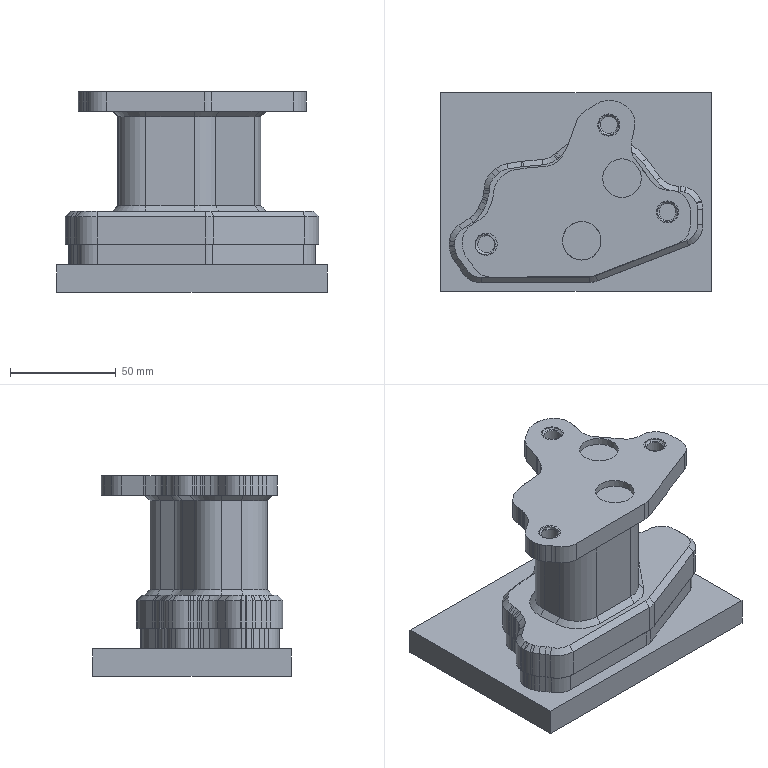NC program | NX | posted by the shop | part box 128.162 x 94.109 x 95 mm
Lines 29924 to 31062 of 131503:
29923 TOOL CALL 12 Z S7000
29924 CALL LBL101
29925 M3 M8
29926 M51
29927 CYCL DEF 32.0 TOLERANCE
29928 CYCL DEF 32.1 T0.036
29929 CYCL DEF 32.2 HSC-MODE:0
29930 L M126
29931 L A+0.0 C+0.0 FMAX
29932 L X15.464 Y31.7104 FMAX
29933 L Z40. FMAX
29934 L Z1. FMAX
29935 CC X15.9765 Y31.7104
29936 C X16.489 Y31.7104 DR+ F1000.
29937 CC X15.464 Y31.7104
29938 CP IPA360. IZ-.2 DR+
29939 CC X15.464 Y31.7104
29940 CP IPA360. IZ-.2 DR+
29941 CC X15.464 Y31.7104
29942 CP IPA360. IZ-.2 DR+
29943 CC X15.464 Y31.7104
29944 CP IPA360. IZ-.2 DR+
29945 CC X15.464 Y31.7104
29946 CP IPA360. IZ-.2 DR+
29947 CC X15.464 Y31.7104
29948 CP IPA360. IZ-.2 DR+
29949 CC X15.464 Y31.7104
29950 CP IPA360. IZ-.2 DR+
29951 CC X15.464 Y31.7104
29952 CP IPA360. IZ-.2 DR+
29953 CC X15.464 Y31.7104
29954 CP IPA360. IZ-.2 DR+
29955 CC X15.464 Y31.7104
29956 CP IPA360. IZ-.2 DR+
29957 CC X15.464 Y31.7104
29958 CP IPA360. IZ-.2 DR+
29959 CC X15.464 Y31.7104
29960 CP IPA360. IZ-.2 DR+
29961 CC X15.464 Y31.7104
29962 CP IPA360. IZ-.2 DR+
29963 CC X15.464 Y31.7104
29964 CP IPA360. IZ-.2 DR+
29965 CC X15.464 Y31.7104
29966 CP IPA360. IZ-.2 DR+
29967 CC X15.464 Y31.7104
29968 CP IPA360. IZ-.2 DR+
29969 CC X15.464 Y31.7104
29970 CP IPA360. IZ-.2 DR+
29971 CC X15.464 Y31.7104
29972 CP IPA360. IZ-.2 DR+
29973 CC X15.464 Y31.7104
29974 CP IPA360. IZ-.2 DR+
29975 CC X15.464 Y31.7104
29976 CP IPA360. IZ-.2 DR+
29977 CC X15.464 Y31.7104
29978 CP IPA360. IZ-.2 DR+
29979 CC X15.464 Y31.7104
29980 CP IPA360. IZ-.2 DR+
29981 CC X15.464 Y31.7104
29982 CP IPA360. IZ-.2 DR+
29983 CC X15.464 Y31.7104
29984 CP IPA360. IZ-.2 DR+
29985 CC X15.464 Y31.7104
29986 CP IPA360. IZ-.2 DR+
29987 CC X15.464 Y31.7104
29988 CP IPA360. IZ-.2 DR+
29989 CC X15.464 Y31.7104
29990 CP IPA360. IZ-.2 DR+
29991 CC X15.464 Y31.7104
29992 CP IPA360. IZ-.2 DR+
29993 CC X15.464 Y31.7104
29994 CP IPA360. IZ-.2 DR+
29995 CC X15.464 Y31.7104
29996 CP IPA360. IZ-.2 DR+
29997 CC X15.464 Y31.7104
29998 CP IPA360. IZ-.2 DR+
29999 CC X15.464 Y31.7104
30000 CP IPA360. IZ-.2 DR+
30001 CC X15.464 Y31.7104
30002 CP IPA360. IZ-.2 DR+
30003 CC X15.464 Y31.7104
30004 CP IPA360. IZ-.2 DR+
30005 CC X15.464 Y31.7104
30006 CP IPA360. IZ-.2 DR+
30007 CC X15.464 Y31.7104
30008 CP IPA360. IZ-.2 DR+
30009 CC X15.464 Y31.7104
30010 CP IPA360. IZ-.2 DR+
30011 CC X15.464 Y31.7104
30012 CP IPA360. IZ-.2 DR+
30013 CC X15.464 Y31.7104
30014 CP IPA360. IZ-.2 DR+
30015 CC X15.464 Y31.7104
30016 CP IPA360. IZ-.2 DR+
30017 CC X15.464 Y31.7104
30018 CP IPA360. IZ-.2 DR+
30019 CC X15.464 Y31.7104
30020 CP IPA360. IZ-.2 DR+
30021 CC X15.464 Y31.7104
30022 CP IPA360. IZ-.2 DR+
30023 CC X15.464 Y31.7104
30024 CP IPA360. IZ-.2 DR+
30025 CC X15.464 Y31.7104
30026 CP IPA360. IZ-.2 DR+
30027 CC X15.464 Y31.7104
30028 CP IPA360. IZ-.2 DR+
30029 CC X15.464 Y31.7104
30030 CP IPA360. IZ-.2 DR+
30031 CC X15.464 Y31.7104
30032 CP IPA360. IZ-.2 DR+
30033 CC X15.464 Y31.7104
30034 CP IPA360. IZ-.2 DR+
30035 CC X15.464 Y31.7104
30036 CP IPA360. IZ-.2 DR+
30037 CC X15.464 Y31.7104
30038 CP IPA360. IZ-.2 DR+
30039 CC X15.464 Y31.7104
30040 CP IPA360. IZ-.2 DR+
30041 CC X15.464 Y31.7104
30042 CP IPA360. IZ-.2 DR+
30043 CC X15.464 Y31.7104
30044 CP IPA360. IZ-.2 DR+
30045 CC X15.464 Y31.7104
30046 CP IPA360. IZ-.2 DR+
30047 CC X15.464 Y31.7104
30048 CP IPA360. IZ-.2 DR+
30049 CC X15.464 Y31.7104
30050 CP IPA217.9924 IZ-.1211 DR+
30051 CC X15.464 Y31.7104
30052 C X14.6562 Y31.0794 DR+
30053 L Z40. FMAX
30054 L X43.2378 Y-9.288 FMAX
30055 L Z1. FMAX
30056 CC X43.7503 Y-9.288
30057 C X44.2628 Y-9.288 DR+
30058 CC X43.2378 Y-9.288
30059 CP IPA360. IZ-.2 DR+
30060 CC X43.2378 Y-9.288
30061 CP IPA360. IZ-.2 DR+
30062 CC X43.2378 Y-9.288
30063 CP IPA360. IZ-.2 DR+
30064 CC X43.2378 Y-9.288
30065 CP IPA360. IZ-.2 DR+
30066 CC X43.2378 Y-9.288
30067 CP IPA360. IZ-.2 DR+
30068 CC X43.2378 Y-9.288
30069 CP IPA360. IZ-.2 DR+
30070 CC X43.2378 Y-9.288
30071 CP IPA360. IZ-.2 DR+
30072 CC X43.2378 Y-9.288
30073 CP IPA360. IZ-.2 DR+
30074 CC X43.2378 Y-9.288
30075 CP IPA360. IZ-.2 DR+
30076 CC X43.2378 Y-9.288
30077 CP IPA360. IZ-.2 DR+
30078 CC X43.2378 Y-9.288
30079 CP IPA360. IZ-.2 DR+
30080 CC X43.2378 Y-9.288
30081 CP IPA360. IZ-.2 DR+
30082 CC X43.2378 Y-9.288
30083 CP IPA360. IZ-.2 DR+
30084 CC X43.2378 Y-9.288
30085 CP IPA360. IZ-.2 DR+
30086 CC X43.2378 Y-9.288
30087 CP IPA360. IZ-.2 DR+
30088 CC X43.2378 Y-9.288
30089 CP IPA360. IZ-.2 DR+
30090 CC X43.2378 Y-9.288
30091 CP IPA360. IZ-.2 DR+
30092 CC X43.2378 Y-9.288
30093 CP IPA360. IZ-.2 DR+
30094 CC X43.2378 Y-9.288
30095 CP IPA360. IZ-.2 DR+
30096 CC X43.2378 Y-9.288
30097 CP IPA360. IZ-.2 DR+
30098 CC X43.2378 Y-9.288
30099 CP IPA360. IZ-.2 DR+
30100 CC X43.2378 Y-9.288
30101 CP IPA360. IZ-.2 DR+
30102 CC X43.2378 Y-9.288
30103 CP IPA360. IZ-.2 DR+
30104 CC X43.2378 Y-9.288
30105 CP IPA360. IZ-.2 DR+
30106 CC X43.2378 Y-9.288
30107 CP IPA360. IZ-.2 DR+
30108 CC X43.2378 Y-9.288
30109 CP IPA360. IZ-.2 DR+
30110 CC X43.2378 Y-9.288
30111 CP IPA360. IZ-.2 DR+
30112 CC X43.2378 Y-9.288
30113 CP IPA360. IZ-.2 DR+
30114 CC X43.2378 Y-9.288
30115 CP IPA360. IZ-.2 DR+
30116 CC X43.2378 Y-9.288
30117 CP IPA360. IZ-.2 DR+
30118 CC X43.2378 Y-9.288
30119 CP IPA360. IZ-.2 DR+
30120 CC X43.2378 Y-9.288
30121 CP IPA360. IZ-.2 DR+
30122 CC X43.2378 Y-9.288
30123 CP IPA360. IZ-.2 DR+
30124 CC X43.2378 Y-9.288
30125 CP IPA360. IZ-.2 DR+
30126 CC X43.2378 Y-9.288
30127 CP IPA360. IZ-.2 DR+
30128 CC X43.2378 Y-9.288
30129 CP IPA360. IZ-.2 DR+
30130 CC X43.2378 Y-9.288
30131 CP IPA360. IZ-.2 DR+
30132 CC X43.2378 Y-9.288
30133 CP IPA360. IZ-.2 DR+
30134 CC X43.2378 Y-9.288
30135 CP IPA360. IZ-.2 DR+
30136 CC X43.2378 Y-9.288
30137 CP IPA360. IZ-.2 DR+
30138 CC X43.2378 Y-9.288
30139 CP IPA360. IZ-.2 DR+
30140 CC X43.2378 Y-9.288
30141 CP IPA360. IZ-.2 DR+
30142 CC X43.2378 Y-9.288
30143 CP IPA360. IZ-.2 DR+
30144 CC X43.2378 Y-9.288
30145 CP IPA360. IZ-.2 DR+
30146 CC X43.2378 Y-9.288
30147 CP IPA360. IZ-.2 DR+
30148 CC X43.2378 Y-9.288
30149 CP IPA360. IZ-.2 DR+
30150 CC X43.2378 Y-9.288
30151 CP IPA360. IZ-.2 DR+
30152 CC X43.2378 Y-9.288
30153 CP IPA360. IZ-.2 DR+
30154 CC X43.2378 Y-9.288
30155 CP IPA360. IZ-.2 DR+
30156 CC X43.2378 Y-9.288
30157 CP IPA360. IZ-.2 DR+
30158 CC X43.2378 Y-9.288
30159 CP IPA360. IZ-.2 DR+
30160 CC X43.2378 Y-9.288
30161 CP IPA360. IZ-.2 DR+
30162 CC X43.2378 Y-9.288
30163 CP IPA360. IZ-.2 DR+
30164 CC X43.2378 Y-9.288
30165 CP IPA360. IZ-.2 DR+
30166 CC X43.2378 Y-9.288
30167 CP IPA360. IZ-.2 DR+
30168 CC X43.2378 Y-9.288
30169 CP IPA360. IZ-.2 DR+
30170 CC X43.2378 Y-9.288
30171 CP IPA217.9924 IZ-.1211 DR+
30172 CC X43.2378 Y-9.288
30173 C X42.43 Y-9.919 DR+
30174 L Z40. FMAX
30175 L X-42.4743 Y-24.6442 FMAX
30176 L Z1. FMAX
30177 CC X-41.9618 Y-24.6442
30178 C X-41.4493 Y-24.6442 DR+
30179 CC X-42.4743 Y-24.6442
30180 CP IPA360. IZ-.2 DR+
30181 CC X-42.4743 Y-24.6442
30182 CP IPA360. IZ-.2 DR+
30183 CC X-42.4743 Y-24.6442
30184 CP IPA360. IZ-.2 DR+
30185 CC X-42.4743 Y-24.6442
30186 CP IPA360. IZ-.2 DR+
30187 CC X-42.4743 Y-24.6442
30188 CP IPA360. IZ-.2 DR+
30189 CC X-42.4743 Y-24.6442
30190 CP IPA360. IZ-.2 DR+
30191 CC X-42.4743 Y-24.6442
30192 CP IPA360. IZ-.2 DR+
30193 CC X-42.4743 Y-24.6442
30194 CP IPA360. IZ-.2 DR+
30195 CC X-42.4743 Y-24.6442
30196 CP IPA360. IZ-.2 DR+
30197 CC X-42.4743 Y-24.6442
30198 CP IPA360. IZ-.2 DR+
30199 CC X-42.4743 Y-24.6442
30200 CP IPA360. IZ-.2 DR+
30201 CC X-42.4743 Y-24.6442
30202 CP IPA360. IZ-.2 DR+
30203 CC X-42.4743 Y-24.6442
30204 CP IPA360. IZ-.2 DR+
30205 CC X-42.4743 Y-24.6442
30206 CP IPA360. IZ-.2 DR+
30207 CC X-42.4743 Y-24.6442
30208 CP IPA360. IZ-.2 DR+
30209 CC X-42.4743 Y-24.6442
30210 CP IPA360. IZ-.2 DR+
30211 CC X-42.4743 Y-24.6442
30212 CP IPA360. IZ-.2 DR+
30213 CC X-42.4743 Y-24.6442
30214 CP IPA360. IZ-.2 DR+
30215 CC X-42.4743 Y-24.6442
30216 CP IPA360. IZ-.2 DR+
30217 CC X-42.4743 Y-24.6442
30218 CP IPA360. IZ-.2 DR+
30219 CC X-42.4743 Y-24.6442
30220 CP IPA360. IZ-.2 DR+
30221 CC X-42.4743 Y-24.6442
30222 CP IPA360. IZ-.2 DR+
30223 CC X-42.4743 Y-24.6442
30224 CP IPA360. IZ-.2 DR+
30225 CC X-42.4743 Y-24.6442
30226 CP IPA360. IZ-.2 DR+
30227 CC X-42.4743 Y-24.6442
30228 CP IPA360. IZ-.2 DR+
30229 CC X-42.4743 Y-24.6442
30230 CP IPA360. IZ-.2 DR+
30231 CC X-42.4743 Y-24.6442
30232 CP IPA360. IZ-.2 DR+
30233 CC X-42.4743 Y-24.6442
30234 CP IPA360. IZ-.2 DR+
30235 CC X-42.4743 Y-24.6442
30236 CP IPA360. IZ-.2 DR+
30237 CC X-42.4743 Y-24.6442
30238 CP IPA360. IZ-.2 DR+
30239 CC X-42.4743 Y-24.6442
30240 CP IPA360. IZ-.2 DR+
30241 CC X-42.4743 Y-24.6442
30242 CP IPA360. IZ-.2 DR+
30243 CC X-42.4743 Y-24.6442
30244 CP IPA360. IZ-.2 DR+
30245 CC X-42.4743 Y-24.6442
30246 CP IPA360. IZ-.2 DR+
30247 CC X-42.4743 Y-24.6442
30248 CP IPA360. IZ-.2 DR+
30249 CC X-42.4743 Y-24.6442
30250 CP IPA360. IZ-.2 DR+
30251 CC X-42.4743 Y-24.6442
30252 CP IPA360. IZ-.2 DR+
30253 CC X-42.4743 Y-24.6442
30254 CP IPA360. IZ-.2 DR+
30255 CC X-42.4743 Y-24.6442
30256 CP IPA360. IZ-.2 DR+
30257 CC X-42.4743 Y-24.6442
30258 CP IPA360. IZ-.2 DR+
30259 CC X-42.4743 Y-24.6442
30260 CP IPA360. IZ-.2 DR+
30261 CC X-42.4743 Y-24.6442
30262 CP IPA360. IZ-.2 DR+
30263 CC X-42.4743 Y-24.6442
30264 CP IPA360. IZ-.2 DR+
30265 CC X-42.4743 Y-24.6442
30266 CP IPA360. IZ-.2 DR+
30267 CC X-42.4743 Y-24.6442
30268 CP IPA360. IZ-.2 DR+
30269 CC X-42.4743 Y-24.6442
30270 CP IPA360. IZ-.2 DR+
30271 CC X-42.4743 Y-24.6442
30272 CP IPA360. IZ-.2 DR+
30273 CC X-42.4743 Y-24.6442
30274 CP IPA360. IZ-.2 DR+
30275 CC X-42.4743 Y-24.6442
30276 CP IPA360. IZ-.2 DR+
30277 CC X-42.4743 Y-24.6442
30278 CP IPA360. IZ-.2 DR+
30279 CC X-42.4743 Y-24.6442
30280 CP IPA360. IZ-.2 DR+
30281 CC X-42.4743 Y-24.6442
30282 CP IPA360. IZ-.2 DR+
30283 CC X-42.4743 Y-24.6442
30284 CP IPA360. IZ-.2 DR+
30285 CC X-42.4743 Y-24.6442
30286 CP IPA360. IZ-.2 DR+
30287 CC X-42.4743 Y-24.6442
30288 CP IPA360. IZ-.2 DR+
30289 CC X-42.4743 Y-24.6442
30290 CP IPA360. IZ-.2 DR+
30291 CC X-42.4743 Y-24.6442
30292 CP IPA217.9924 IZ-.1211 DR+
30293 CC X-42.4743 Y-24.6442
30294 C X-43.2821 Y-25.2752 DR+
30295 L Z40. FMAX
30296 PLANE RESET STAY
30297 * - OPERATION: 精小孔-1 - TOOL: T12 J-D4
30298 CYCL DEF 32.0 TOLERANCE
30299 CYCL DEF 32.1 T0.001
30300 CYCL DEF 32.2 HSC-MODE:0
30301 L A+0.0 C+0.0 FMAX
30302 L X-41.5872 Y-24.7754 FMAX
30303 L Z40. FMAX
30304 L Z-5. FMAX
30305 L Z-6. F250.
30306 L X-41.4932 Y-24.8096 RL
30307 L X-41.4126 Y-24.8238
30308 CC X-41.3952 Y-24.7253
30309 C X-41.2967 Y-24.7427 DR+
30310 L X-41.2793 Y-24.6442
30311 CC X-42.4743 Y-24.6442
30312 C X-41.2793 Y-24.6442 DR+ F200.
30313 CC X-42.4743 Y-24.6442
30314 C X-41.2795 Y-24.6242 DR+
30315 CC X-41.3795 Y-24.6259
30316 C X-41.3812 Y-24.5259 DR+
30317 L X-41.4793 Y-24.5449 R0
30318 L X-41.4778 Y-24.7269
30319 L X-41.3793 Y-24.7442 RL F250.
30320 CC X-41.3793 Y-24.6442
30321 C X-41.2793 Y-24.6442 DR+
30322 CC X-42.4743 Y-24.6442
30323 C X-41.2793 Y-24.6442 DR+ F200.
30324 CC X-42.4743 Y-24.6442
30325 C X-41.2795 Y-24.6242 DR+
30326 CC X-41.3795 Y-24.6259
30327 C X-41.3812 Y-24.5259 DR+
30328 L X-41.4862 Y-24.5277
30329 L X-41.5844 Y-24.5467 R0
30330 L Z-5.
30331 L Z40. FMAX
30332 L X-41.5829 Y-24.7269 FMAX
30333 L Z-10.3211 FMAX
30334 L Z-11.3211 F250.
30335 L X-41.4844 Y-24.7442 RL
30336 L X-41.3793
30337 CC X-41.3793 Y-24.6442
30338 C X-41.2793 Y-24.6442 DR+
30339 CC X-42.4743 Y-24.6442
30340 C X-41.2793 Y-24.6442 DR+ F200.
30341 CC X-42.4743 Y-24.6442
30342 C X-41.2795 Y-24.6242 DR+
30343 CC X-41.3795 Y-24.6259
30344 C X-41.3812 Y-24.5259 DR+
30345 L X-41.4793 Y-24.5449 R0
30346 L X-41.4778 Y-24.7269
30347 L X-41.3793 Y-24.7442 RL F250.
30348 CC X-41.3793 Y-24.6442
30349 C X-41.2793 Y-24.6442 DR+
30350 CC X-42.4743 Y-24.6442
30351 C X-41.2793 Y-24.6442 DR+ F200.
30352 CC X-42.4743 Y-24.6442
30353 C X-41.2795 Y-24.6242 DR+
30354 CC X-41.3795 Y-24.6259
30355 C X-41.3812 Y-24.5259 DR+
30356 L X-41.4862 Y-24.5277
30357 L X-41.5844 Y-24.5467 R0
30358 L Z-10.3211
30359 L Z40. FMAX
30360 L X16.3554 Y31.6277 FMAX
30361 L Z-5. FMAX
30362 L Z-6. F250.
30363 L X16.4539 Y31.6104 RL
30364 L X16.559
30365 CC X16.559 Y31.7104
30366 C X16.659 Y31.7104 DR+
30367 CC X15.464 Y31.7104
30368 C X16.659 Y31.7104 DR+ F200.
30369 CC X15.464 Y31.7104
30370 C X16.6588 Y31.7304 DR+
30371 CC X16.5588 Y31.7287
30372 C X16.5571 Y31.8287 DR+
30373 L X16.459 Y31.8097 R0
30374 L X16.4605 Y31.6277
30375 L X16.559 Y31.6104 RL F250.
30376 CC X16.559 Y31.7104
30377 C X16.659 Y31.7104 DR+
30378 CC X15.464 Y31.7104
30379 C X16.659 Y31.7104 DR+ F200.
30380 CC X15.464 Y31.7104
30381 C X16.6588 Y31.7304 DR+
30382 CC X16.5588 Y31.7287
30383 C X16.5571 Y31.8287 DR+
30384 L X16.4521 Y31.8269
30385 L X16.3539 Y31.8079 R0
30386 L Z-5.
30387 L Z40. FMAX
30388 L X16.3554 Y31.6277 FMAX
30389 L Z-10.3211 FMAX
30390 L Z-11.3211 F250.
30391 L X16.4539 Y31.6104 RL
30392 L X16.559
30393 CC X16.559 Y31.7104
30394 C X16.659 Y31.7104 DR+
30395 CC X15.464 Y31.7104
30396 C X16.659 Y31.7104 DR+ F200.
30397 CC X15.464 Y31.7104
30398 C X16.6588 Y31.7304 DR+
30399 CC X16.5588 Y31.7287
30400 C X16.5571 Y31.8287 DR+
30401 L X16.459 Y31.8097 R0
30402 L X16.4605 Y31.6277
30403 L X16.559 Y31.6104 RL F250.
30404 CC X16.559 Y31.7104
30405 C X16.659 Y31.7104 DR+
30406 CC X15.464 Y31.7104
30407 C X16.659 Y31.7104 DR+ F200.
30408 CC X15.464 Y31.7104
30409 C X16.6588 Y31.7304 DR+
30410 CC X16.5588 Y31.7287
30411 C X16.5571 Y31.8287 DR+
30412 L X16.4521 Y31.8269
30413 L X16.3539 Y31.8079 R0
30414 L Z-10.3211
30415 L Z40. FMAX
30416 L X44.1292 Y-9.3707 FMAX
30417 L Z-5. FMAX
30418 L Z-6. F250.
30419 L X44.2277 Y-9.388 RL
30420 L X44.3328
30421 CC X44.3328 Y-9.288
30422 C X44.4328 Y-9.288 DR+
30423 CC X43.2378 Y-9.288
30424 C X44.4328 Y-9.288 DR+ F200.
30425 CC X43.2378 Y-9.288
30426 C X44.4326 Y-9.268 DR+
30427 CC X44.3326 Y-9.2697
30428 C X44.3309 Y-9.1697 DR+
30429 L X44.2328 Y-9.1887 R0
30430 L X44.2343 Y-9.3707
30431 L X44.3328 Y-9.388 RL F250.
30432 CC X44.3328 Y-9.288
30433 C X44.4328 Y-9.288 DR+
30434 CC X43.2378 Y-9.288
30435 C X44.4328 Y-9.288 DR+ F200.
30436 CC X43.2378 Y-9.288
30437 C X44.4326 Y-9.268 DR+
30438 CC X44.3326 Y-9.2697
30439 C X44.3309 Y-9.1697 DR+
30440 L X44.2259 Y-9.1715
30441 L X44.1277 Y-9.1905 R0
30442 L Z-5.
30443 L Z40. FMAX
30444 L X44.1292 Y-9.3707 FMAX
30445 L Z-10.3211 FMAX
30446 L Z-11.3211 F250.
30447 L X44.2277 Y-9.388 RL
30448 L X44.3328
30449 CC X44.3328 Y-9.288
30450 C X44.4328 Y-9.288 DR+
30451 CC X43.2378 Y-9.288
30452 C X44.4328 Y-9.288 DR+ F200.
30453 CC X43.2378 Y-9.288
30454 C X44.4326 Y-9.268 DR+
30455 CC X44.3326 Y-9.2697
30456 C X44.3309 Y-9.1697 DR+
30457 L X44.2328 Y-9.1887 R0
30458 L X44.2343 Y-9.3707
30459 L X44.3328 Y-9.388 RL F250.
30460 CC X44.3328 Y-9.288
30461 C X44.4328 Y-9.288 DR+
30462 CC X43.2378 Y-9.288
30463 C X44.4328 Y-9.288 DR+ F200.
30464 CC X43.2378 Y-9.288
30465 C X44.4326 Y-9.268 DR+
30466 CC X44.3326 Y-9.2697
30467 C X44.3309 Y-9.1697 DR+
30468 L X44.2259 Y-9.1715
30469 L X44.1277 Y-9.1905 R0
30470 L Z-10.3211
30471 L Z40. FMAX
30472 PLANE RESET STAY
30473 M50
30474 * - OPERATION: 精飞平面_1 - TOOL: T15 J-D10
30475 M5
30476 M9
30477 PLANE RESET STAY
30478 CALL LBL100
30479 ;(J-D10 D=10. R=0.)
30480 M01
30481 TOOL CALL 15 Z S7000
30482 CALL LBL101
30483 M3 M8
30484 M51
30485 CYCL DEF 32.0 TOLERANCE
30486 CYCL DEF 32.1 T0.036
30487 CYCL DEF 32.2 HSC-MODE:0
30488 L M126
30489 L A+0.0 C+0.0 FMAX
30490 L X31.226 Y-37.6718 FMAX
30491 L Z43. FMAX
30492 L Z3. FMAX
30493 L Z+0.0 F700.
30494 L X28.175
30495 L X-53.175
30496 L X-55.4397 Y-34.4703
30497 L X-56.355 Y-33.1485
30498 L X-57.1186 Y-31.7337
30499 L X-57.7212 Y-30.2431
30500 L X-57.8456 Y-29.8785
30501 L X48.3375
30502 L X49.8598 Y-29.2901
30503 CC X44.6231 Y-15.7419
30504 C X57.6898 Y-22.0852 DR+
30505 L X-58.7822
30506 CC X-44.3628 Y-23.8354
30507 C X-58.7587 Y-21.9016 DR-
30508 CC X-44.3542 Y-23.7687
30509 C X-55.3617 Y-14.2918 DR-
30510 L X59.1481
30511 L Y-9.2928
30512 CC X44.6231 Y-9.2928
30513 C X58.8768 Y-6.4985 DR+
30514 L X-45.9534
30515 L X-43.8624 Y1.2948
30516 L X54.8204
30517 L X53.6659 Y2.3471
30518 L X52.4051 Y3.2693
30519 L X51.0526 Y4.0508
30520 L X49.6239 Y4.6825
30521 L X38.8425 Y9.0881
30522 L X-40.2677
30523 CC X-29.4643 Y-.6208
30524 C X-38.9932 Y10.3417 DR-
30525 L X-37.2409 Y11.8648
30526 CC X-27.7121 Y.9023
30527 C X-29.9026 Y15.2611 DR-
30528 L X-23.8929 Y16.178
30529 CC X-21.7023 Y1.8191
30530 C X-22.9249 Y16.2926 DR-
30531 L X-15.9541 Y16.8814
30532 L X32.9578
30533 L X31.5734 Y24.6747
30534 L X-8.1136
30535 L X-5.3425 Y32.4681
30536 L X32.8357
30537 CC X18.3114 Y32.6039
30538 C X30.6539 Y40.2614 DR+
30539 L X-1.0929
30540 L X-2.5945
30541 L Z3.
30542 L Z43. FMAX
30543 PLANE RESET STAY
30544 * - OPERATION: 精大孔-1 - TOOL: T15 J-D10
30545 CYCL DEF 32.0 TOLERANCE
30546 CYCL DEF 32.1 T0.001
30547 CYCL DEF 32.2 HSC-MODE:0
30548 L A+0.0 C+0.0 FMAX
30549 L X5.5902 Y-24.1174 FMAX
30550 L Z40. FMAX
30551 L Z-2.3481 FMAX
30552 L Z-3.3481 F250.
30553 L X5.6842 Y-24.1516 RL
30554 L X5.7433 Y-24.162
30555 CC X5.9169 Y-23.1772
30556 C X6.9017 Y-23.3508 DR+
30557 L X6.9191 Y-23.2524
30558 CC X2.7551 Y-23.2524
30559 C X6.9191 Y-23.2524 DR+ F400.
30560 CC X2.7551 Y-23.2524
30561 C X6.8891 Y-22.7536 DR+
30562 CC X5.8963 Y-22.8733
30563 C X5.7765 Y-21.8805 DR+
30564 L X5.6808 Y-21.9096 R0
30565 L X5.8206 Y-24.235
30566 L X5.9191 Y-24.2524 RL F250.
30567 CC X5.9191 Y-23.2524
30568 C X6.9191 Y-23.2524 DR+
30569 CC X2.7551 Y-23.2524
30570 C X6.9191 Y-23.2524 DR+ F400.
30571 CC X2.7551 Y-23.2524
30572 C X6.8891 Y-22.7536 DR+
30573 CC X5.8963 Y-22.8733
30574 C X5.7765 Y-21.8805 DR+
30575 L X5.5107 Y-21.9126
30576 L X5.415 Y-21.9417 R0
30577 L Z-2.3481
30578 L Z40. FMAX
30579 L X24.5725 Y5.4185 FMAX
30580 L Z-2.3481 FMAX
30581 L Z-3.3481 F250.
30582 L X24.671 Y5.4011 RL
30583 L X24.9388
30584 CC X24.9388 Y6.4011
30585 C X25.9388 Y6.4011 DR+
30586 CC X21.7748 Y6.4011
30587 C X25.9388 Y6.4011 DR+ F400.
30588 CC X21.7748 Y6.4011
30589 C X25.9088 Y6.8999 DR+
30590 CC X24.916 Y6.7801
30591 C X24.7962 Y7.7729 DR+
30592 L X24.7005 Y7.7439 R0
30593 L X24.8403 Y5.4185
30594 L X24.9388 Y5.4011 RL F250.
30595 CC X24.9388 Y6.4011
30596 C X25.9388 Y6.4011 DR+
30597 CC X21.7748 Y6.4011
30598 C X25.9388 Y6.4011 DR+ F400.
30599 CC X21.7748 Y6.4011
30600 C X25.9088 Y6.8999 DR+
30601 CC X24.916 Y6.7801
30602 C X24.7962 Y7.7729 DR+
30603 L X24.5304 Y7.7409
30604 L X24.4347 Y7.7118 R0
30605 L Z-2.3481
30606 L Z40. FMAX
30607 PLANE RESET STAY
30608 * - OPERATION: 精大孔-1_COPY - TOOL: T15 J-D10
30609 CYCL DEF 32.0 TOLERANCE
30610 CYCL DEF 32.1 T0.001
30611 CYCL DEF 32.2 HSC-MODE:0
30612 L A+0.0 C+0.0 FMAX
30613 L X-16.2893 Y-46.5602 FMAX
30614 L Z40. FMAX
30615 L Z-13.3211 FMAX
30616 L Z-14.3211 F250.
30617 L X-16.2628 Y-46.4638 RL
30618 CC X-17.2584 Y-46.3701
30619 C X-17.0889 Y-45.3846 DR+
30620 L X-17.1875 Y-45.3677
30621 L X-40.2428 Y-45.465 F400.
30622 CC X-40.3041 Y-30.9401
30623 C X-53.3634 Y-37.2985 DR-
30624 CC X-57.4318 Y-39.2794
30625 C X-53.86 Y-36.5013 DR+
30626 L X-55.4397 Y-34.4703
30627 CC X-43.9743 Y-25.5528
30628 C X-57.7212 Y-30.2431 DR-
30629 L X-58.068 Y-29.2265
30630 CC X-44.3212 Y-24.5362
30631 C X-58.8153 Y-25.4831 DR-
30632 L X-58.8597 Y-24.8033
30633 CC X-44.3656 Y-23.8564
30634 C X-58.7701 Y-21.9893 DR-
30635 L X-58.7587 Y-21.9016
30636 CC X-44.3542 Y-23.7687
30637 C X-52.3235 Y-11.6251 DR-
30638 L X-47.6587 Y-8.5639
30639 CC X-50.1413 Y-4.7807
30640 C X-46.0013 Y-6.6072 DR+
30641 L X-44.8266 Y-3.9445
30642 CC X-48.9666 Y-2.118
30643 C X-44.6359 Y-3.4297 DR+
30644 L X-44.3352 Y-2.4369
30645 CC X-48.6659 Y-1.1252
30646 C X-44.1785 Y-1.7069 DR+
30647 L X-44.0103 Y-.4097
30648 CC X-48.4978 Y.172
30649 C X-43.9767 Y-.0163 DR+
30650 CC X-29.4643 Y-.6208
30651 C X-38.9932 Y10.3417 DR-
30652 L X-37.2409 Y11.8648
30653 CC X-27.7121 Y.9023
30654 C X-29.9026 Y15.2611 DR-
30655 L X-23.8929 Y16.178
30656 CC X-21.7023 Y1.8191
30657 C X-22.9249 Y16.2926 DR-
30658 L X-14.7012 Y16.9873
30659 CC X-15.0821 Y21.4962
30660 C X-12.3142 Y17.9165 DR+
30661 L X-11.9204 Y18.2209
30662 CC X-14.6883 Y21.8007
30663 C X-10.6782 Y19.7044 DR+
30664 L X-8.3272 Y24.2019
30665 CC X-12.3374 Y26.2981
30666 C X-8.0736 Y24.7829 DR+
30667 L X-4.4864 Y34.8768
30668 CC X9.2 Y30.0129
30669 C X1.5405 Y42.3542 DR-
30670 L X7.1779 Y45.853
30671 CC X14.8374 Y33.5117
30672 C X13.9626 Y48.0103 DR-
30673 L X14.2609 Y48.0283
30674 CC X15.1357 Y33.5297
30675 C X15.1357 Y48.0547 DR-
30676 L X16.7996
30677 CC X16.7996 Y33.5297
30678 C X18.1505 Y47.9917 DR-
30679 L X18.2739 Y47.9802
30680 CC X16.9231 Y33.5182
30681 C X24.2875 Y46.0378 DR-
30682 L X25.5374 Y45.3025
30683 CC X18.1729 Y32.7829
30684 C X29.6636 Y41.6677 DR-
30685 L X29.8021 Y41.4887
30686 CC X18.3114 Y32.6039
30687 C X32.7198 Y30.7677 DR-
30688 L X32.4051 Y28.2978
30689 CC X17.9966 Y30.1341
30690 C X32.0312 Y26.3915 DR-
30691 L X31.2252 Y23.3692
30692 CC X35.5975 Y22.2033
30693 C X31.0725 Y22.2033 DR+
30694 L Y21.1031
30695 CC X35.5975 Y21.1031
30696 C X31.1481 Y20.2791 DR+
30697 L X31.1992 Y20.0031
30698 CC X35.6486 Y20.8271
30699 C X32.0374 Y18.1003 DR+
30700 L X40.0859 Y7.4414
30701 CC X43.6971 Y10.1682
30702 C X43.6971 Y5.6432 DR+
30703 L X44.4097
30704 CC X44.4097 Y-8.8818
30705 C X48.1522 Y5.1528 DR-
30706 L X48.2153 Y5.1359
30707 CC X44.4728 Y-8.8986
30708 C X58.0442 Y-3.7226 DR-
30709 L X58.1945 Y-4.1167
30710 CC X44.6231 Y-9.2928
30711 C X59.1481 Y-9.2928 DR-
30712 L Y-15.7419
30713 CC X44.6231 Y-15.7419
30714 C X49.8598 Y-29.2901 DR-
30715 L X11.0432 Y-44.2936
30716 CC X5.8065 Y-30.7455
30717 C X5.8678 Y-45.2703 DR-
30718 L X-17.1875 Y-45.3677
30719 L X-17.6875 Y-45.3698
30720 CC X-17.6832 Y-46.3698
30721 C X-18.6832 Y-46.374 DR+
30722 L X-18.6654 Y-46.4724 R0
30723 L X-16.2002 Y-46.462
30724 L X-16.1832 Y-46.3634 RL F250.
30725 CC X-17.1832 Y-46.3677
30726 C X-17.1875 Y-45.3677 DR+
30727 L X-40.2428 Y-45.465 F400.
30728 CC X-40.3041 Y-30.9401
30729 C X-53.3634 Y-37.2985 DR-
30730 CC X-57.4318 Y-39.2794
30731 C X-53.86 Y-36.5013 DR+
30732 L X-55.4397 Y-34.4703
30733 CC X-43.9743 Y-25.5528
30734 C X-57.7212 Y-30.2431 DR-
30735 L X-58.068 Y-29.2265
30736 CC X-44.3212 Y-24.5362
30737 C X-58.8153 Y-25.4831 DR-
30738 L X-58.8597 Y-24.8033
30739 CC X-44.3656 Y-23.8564
30740 C X-58.7701 Y-21.9893 DR-
30741 L X-58.7587 Y-21.9016
30742 CC X-44.3542 Y-23.7687
30743 C X-52.3235 Y-11.6251 DR-
30744 L X-47.6587 Y-8.5639
30745 CC X-50.1413 Y-4.7807
30746 C X-46.0013 Y-6.6072 DR+
30747 L X-44.8266 Y-3.9445
30748 CC X-48.9666 Y-2.118
30749 C X-44.6359 Y-3.4297 DR+
30750 L X-44.3352 Y-2.4369
30751 CC X-48.6659 Y-1.1252
30752 C X-44.1785 Y-1.7069 DR+
30753 L X-44.0103 Y-.4097
30754 CC X-48.4978 Y.172
30755 C X-43.9767 Y-.0163 DR+
30756 CC X-29.4643 Y-.6208
30757 C X-38.9932 Y10.3417 DR-
30758 L X-37.2409 Y11.8648
30759 CC X-27.7121 Y.9023
30760 C X-29.9026 Y15.2611 DR-
30761 L X-23.8929 Y16.178
30762 CC X-21.7023 Y1.8191
30763 C X-22.9249 Y16.2926 DR-
30764 L X-14.7012 Y16.9873
30765 CC X-15.0821 Y21.4962
30766 C X-12.3142 Y17.9165 DR+
30767 L X-11.9204 Y18.2209
30768 CC X-14.6883 Y21.8007
30769 C X-10.6782 Y19.7044 DR+
30770 L X-8.3272 Y24.2019
30771 CC X-12.3374 Y26.2981
30772 C X-8.0736 Y24.7829 DR+
30773 L X-4.4864 Y34.8768
30774 CC X9.2 Y30.0129
30775 C X1.5405 Y42.3542 DR-
30776 L X7.1779 Y45.853
30777 CC X14.8374 Y33.5117
30778 C X13.9626 Y48.0103 DR-
30779 L X14.2609 Y48.0283
30780 CC X15.1357 Y33.5297
30781 C X15.1357 Y48.0547 DR-
30782 L X16.7996
30783 CC X16.7996 Y33.5297
30784 C X18.1505 Y47.9917 DR-
30785 L X18.2739 Y47.9802
30786 CC X16.9231 Y33.5182
30787 C X24.2875 Y46.0378 DR-
30788 L X25.5374 Y45.3025
30789 CC X18.1729 Y32.7829
30790 C X29.6636 Y41.6677 DR-
30791 L X29.8021 Y41.4887
30792 CC X18.3114 Y32.6039
30793 C X32.7198 Y30.7677 DR-
30794 L X32.4051 Y28.2978
30795 CC X17.9966 Y30.1341
30796 C X32.0312 Y26.3915 DR-
30797 L X31.2252 Y23.3692
30798 CC X35.5975 Y22.2033
30799 C X31.0725 Y22.2033 DR+
30800 L Y21.1031
30801 CC X35.5975 Y21.1031
30802 C X31.1481 Y20.2791 DR+
30803 L X31.1992 Y20.0031
30804 CC X35.6486 Y20.8271
30805 C X32.0374 Y18.1003 DR+
30806 L X40.0859 Y7.4414
30807 CC X43.6971 Y10.1682
30808 C X43.6971 Y5.6432 DR+
30809 L X44.4097
30810 CC X44.4097 Y-8.8818
30811 C X48.1522 Y5.1528 DR-
30812 L X48.2153 Y5.1359
30813 CC X44.4728 Y-8.8986
30814 C X58.0442 Y-3.7226 DR-
30815 L X58.1945 Y-4.1167
30816 CC X44.6231 Y-9.2928
30817 C X59.1481 Y-9.2928 DR-
30818 L Y-15.7419
30819 CC X44.6231 Y-15.7419
30820 C X49.8598 Y-29.2901 DR-
30821 L X11.0432 Y-44.2936
30822 CC X5.8065 Y-30.7455
30823 C X5.8678 Y-45.2703 DR-
30824 L X-17.1875 Y-45.3677
30825 L X-17.6875 Y-45.3698
30826 CC X-17.6832 Y-46.3698
30827 C X-18.6832 Y-46.374 DR+
30828 L X-18.6828 Y-46.474
30829 L X-18.665 Y-46.5724 R0
30830 L Z-13.3211
30831 L Z40. FMAX
30832 PLANE RESET STAY
30833 M50
30834 * - OPERATION: 精大孔-1_COPY_COPY - TOOL: T16 J-D16
30835 M5
30836 M9
30837 PLANE RESET STAY
30838 CALL LBL100
30839 ;(J-D16 D=16. R=0.)
30840 M01
30841 TOOL CALL 16 Z S2000
30842 CALL LBL101
30843 M3 M8
30844 M51
30845 CYCL DEF 32.0 TOLERANCE
30846 CYCL DEF 32.1 T0.001
30847 CYCL DEF 32.2 HSC-MODE:0
30848 L M126
30849 L A+0.0 C+0.0 FMAX
30850 L X-18.3508 Y-52.1388 FMAX
30851 L Z40. FMAX
30852 L Z-71.4361 FMAX
30853 L Z-72.4361 F250.
30854 L X-18.3243 Y-52.0424 RL
30855 CC X-19.3199 Y-51.9488
30856 C X-19.1504 Y-50.9632 DR+
30857 L X-19.249 Y-50.9463
30858 L X-44.8913 Y-51.0545 F400.
30859 CC X-44.9698 Y-32.4609
30860 C X-61.6874 Y-40.6004 DR-
30861 CC X-64.0194 Y-41.7359
30862 C X-61.972 Y-40.1434 DR+
30863 L X-63.7289 Y-37.8845
30864 CC X-49.0519 Y-26.4691
30865 C X-66.6496 Y-32.4732 DR-
30866 L X-67.0354 Y-31.3425
30867 CC X-49.4377 Y-25.3384
30868 C X-67.9919 Y-26.5506 DR-
30869 L X-68.0413 Y-25.7945
30870 CC X-49.4871 Y-24.5823
30871 C X-67.9266 Y-22.1922 DR-
30872 L X-67.914 Y-22.0947
30873 CC X-49.4744 Y-24.4848
30874 C X-59.676 Y-8.9395 DR-
30875 L X-54.4878 Y-5.5347
30876 CC X-55.9109 Y-3.3662
30877 C X-53.5378 Y-4.4131 DR+
30878 L X-52.2312 Y-1.4516
30879 CC X-54.6044 Y-.4047
30880 C X-52.1219 Y-1.1565 DR+
30881 L X-51.7875 Y-.0523
30882 CC X-54.2699 Y.6995
30883 C X-51.6977 Y.3661 DR+
30884 L X-51.5106 Y1.8089
30885 CC X-54.0829 Y2.1423
30886 C X-51.4914 Y2.0343 DR+
30887 CC X-32.9137 Y1.2606
30888 C X-45.1118 Y15.2939 DR-
30889 L X-43.163 Y16.9879
30890 CC X-30.9648 Y2.9545
30891 C X-33.769 Y21.3357 DR-
30892 L X-27.0849 Y22.3554
30893 CC X-24.2807 Y3.9743
30894 C X-25.8458 Y22.5021 DR-
30895 L X-16.6993 Y23.2747
30896 CC X-16.9177 Y25.8593
30897 C X-15.3311 Y23.8074 DR+
30898 L X-14.8931 Y24.146
30899 CC X-16.4797 Y26.1979
30900 C X-14.6803 Y24.3298 DR+
30901 CC X9.3718 Y-.6402
30902 C X-10.0974 Y28.047 DR-
30903 L X-7.3132 Y35.8814
30904 CC X9.2 Y30.0129
30905 C X-.0415 Y44.9032 DR-
30906 L X5.5959 Y48.402
30907 CC X14.8374 Y33.5117
30908 C X13.7819 Y51.0049 DR-
30909 L X14.0802 Y51.0229
30910 CC X15.1357 Y33.5297
30911 C X15.1357 Y51.0547 DR-
30912 L X16.7996
30913 CC X16.7996 Y33.5297
30914 C X18.4295 Y50.9787 DR-
30915 L X18.5529 Y50.9672
30916 CC X16.9231 Y33.5182
30917 C X25.8086 Y48.6236 DR-
30918 L X27.0585 Y47.8883
30919 CC X18.1729 Y32.7829
30920 C X32.0369 Y43.5028 DR-
30921 L X32.1754 Y43.3237
30922 CC X18.3114 Y32.6039
30923 C X35.6958 Y30.3884 DR-
30924 L X35.381 Y27.9186
30925 CC X17.9966 Y30.1341
30926 C X34.9515 Y25.7005 DR-
30927 CC X11.9727 Y-.2607
30928 C X39.6408 Y20.6315 DR-
30929 L X46.3871 Y11.6972
30930 CC X48.4571 Y13.2602
30931 C X48.4571 Y10.6664 DR+
30932 L X49.2496
30933 CC X49.2496 Y-7.9274
30934 C X54.0406 Y10.0386 DR-
30935 L X54.1108 Y10.0199
30936 CC X49.3199 Y-7.9461
30937 C X66.693 Y-1.3201 DR-
30938 L X66.8602 Y-1.7585
30939 CC X49.4871 Y-8.3845
30940 C X68.0809 Y-8.3845 DR-
30941 L Y-15.5573
30942 CC X49.4871 Y-15.5573
30943 C X56.1907 Y-32.9006 DR-
30944 L X13.0185 Y-49.5877
30945 CC X6.3149 Y-32.2444
30946 C X6.3934 Y-50.838 DR-
30947 L X-19.249 Y-50.9463
30948 L X-19.749 Y-50.9484
30949 CC X-19.7447 Y-51.9484
30950 C X-20.7447 Y-51.9526 DR+
30951 L X-20.727 Y-52.051 R0
30952 L X-18.2617 Y-52.0406
30953 L X-18.2448 Y-51.9421 RL F250.
30954 CC X-19.2448 Y-51.9463
30955 C X-19.249 Y-50.9463 DR+
30956 L X-44.8913 Y-51.0545 F400.
30957 CC X-44.9698 Y-32.4609
30958 C X-61.6874 Y-40.6004 DR-
30959 CC X-64.0194 Y-41.7359
30960 C X-61.972 Y-40.1434 DR+
30961 L X-63.7289 Y-37.8845
30962 CC X-49.0519 Y-26.4691
30963 C X-66.6496 Y-32.4732 DR-
30964 L X-67.0354 Y-31.3425
30965 CC X-49.4377 Y-25.3384
30966 C X-67.9919 Y-26.5506 DR-
30967 L X-68.0413 Y-25.7945
30968 CC X-49.4871 Y-24.5823
30969 C X-67.9266 Y-22.1922 DR-
30970 L X-67.914 Y-22.0947
30971 CC X-49.4744 Y-24.4848
30972 C X-59.676 Y-8.9395 DR-
30973 L X-54.4878 Y-5.5347
30974 CC X-55.9109 Y-3.3662
30975 C X-53.5378 Y-4.4131 DR+
30976 L X-52.2312 Y-1.4516
30977 CC X-54.6044 Y-.4047
30978 C X-52.1219 Y-1.1565 DR+
30979 L X-51.7875 Y-.0523
30980 CC X-54.2699 Y.6995
30981 C X-51.6977 Y.3661 DR+
30982 L X-51.5106 Y1.8089
30983 CC X-54.0829 Y2.1423
30984 C X-51.4914 Y2.0343 DR+
30985 CC X-32.9137 Y1.2606
30986 C X-45.1118 Y15.2939 DR-
30987 L X-43.163 Y16.9879
30988 CC X-30.9648 Y2.9545
30989 C X-33.769 Y21.3357 DR-
30990 L X-27.0849 Y22.3554
30991 CC X-24.2807 Y3.9743
30992 C X-25.8458 Y22.5021 DR-
30993 L X-16.6993 Y23.2747
30994 CC X-16.9177 Y25.8593
30995 C X-15.3311 Y23.8074 DR+
30996 L X-14.8931 Y24.146
30997 CC X-16.4797 Y26.1979
30998 C X-14.6803 Y24.3298 DR+
30999 CC X9.3718 Y-.6402
31000 C X-10.0974 Y28.047 DR-
31001 L X-7.3132 Y35.8814
31002 CC X9.2 Y30.0129
31003 C X-.0415 Y44.9032 DR-
31004 L X5.5959 Y48.402
31005 CC X14.8374 Y33.5117
31006 C X13.7819 Y51.0049 DR-
31007 L X14.0802 Y51.0229
31008 CC X15.1357 Y33.5297
31009 C X15.1357 Y51.0547 DR-
31010 L X16.7996
31011 CC X16.7996 Y33.5297
31012 C X18.4295 Y50.9787 DR-
31013 L X18.5529 Y50.9672
31014 CC X16.9231 Y33.5182
31015 C X25.8086 Y48.6236 DR-
31016 L X27.0585 Y47.8883
31017 CC X18.1729 Y32.7829
31018 C X32.0369 Y43.5028 DR-
31019 L X32.1754 Y43.3237
31020 CC X18.3114 Y32.6039
31021 C X35.6958 Y30.3884 DR-
31022 L X35.381 Y27.9186
31023 CC X17.9966 Y30.1341
31024 C X34.9515 Y25.7005 DR-
31025 CC X11.9727 Y-.2607
31026 C X39.6408 Y20.6315 DR-
31027 L X46.3871 Y11.6972
31028 CC X48.4571 Y13.2602
31029 C X48.4571 Y10.6664 DR+
31030 L X49.2496
31031 CC X49.2496 Y-7.9274
31032 C X54.0406 Y10.0386 DR-
31033 L X54.1108 Y10.0199
31034 CC X49.3199 Y-7.9461
31035 C X66.693 Y-1.3201 DR-
31036 L X66.8602 Y-1.7585
31037 CC X49.4871 Y-8.3845
31038 C X68.0809 Y-8.3845 DR-
31039 L Y-15.5573
31040 CC X49.4871 Y-15.5573
31041 C X56.1907 Y-32.9006 DR-
31042 L X13.0185 Y-49.5877
31043 CC X6.3149 Y-32.2444
31044 C X6.3934 Y-50.838 DR-
31045 L X-19.249 Y-50.9463
31046 L X-19.749 Y-50.9484
31047 CC X-19.7447 Y-51.9484
31048 C X-20.7447 Y-51.9526 DR+
31049 L X-20.7443 Y-52.0526
31050 L X-20.7265 Y-52.151 R0
31051 L Z-71.4361
31052 L Z40. FMAX
31053 PLANE RESET STAY
31054 M50
31055 * - OPERATION: 新底壁铣_1 - TOOL: T10 J-D6R0.5
31056 M5
31057 M9
31058 PLANE RESET STAY
31059 CALL LBL100
31060 ;(J-D6R0.5 D=6. R=0.5)
31061 M01